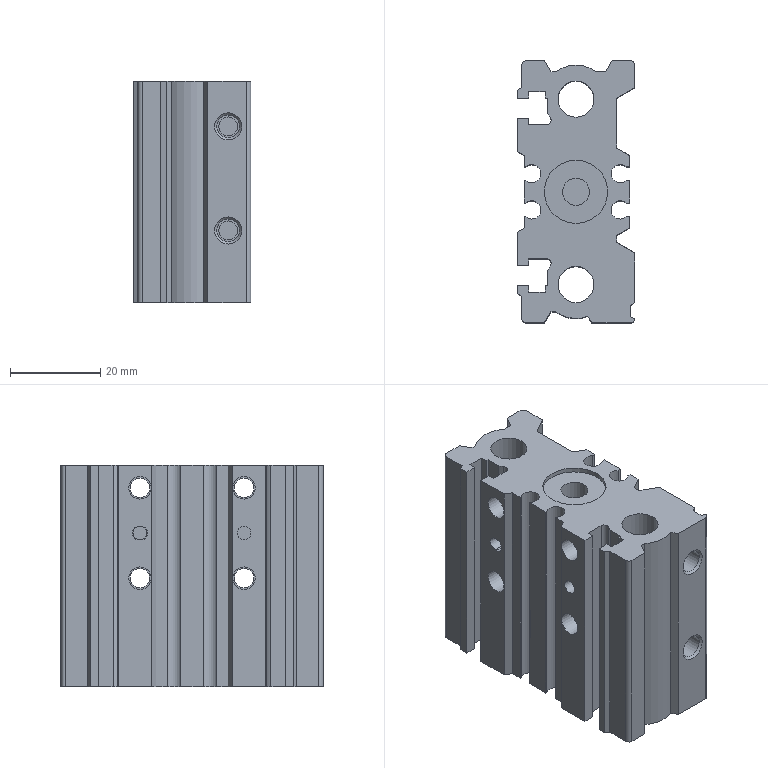Part | STEP file | ROTATION MC_NEW VER-0610_494 | 1 solid | 571 faces | box 26 x 58 x 49 mm | volume 47669 mm3 | plane 349 | spline 166 | cylinder 52 | cone 4 | commonest cylinder face diameters 3 x8 5 x8 2 x6 8 x6 4 x4 4.05 x4